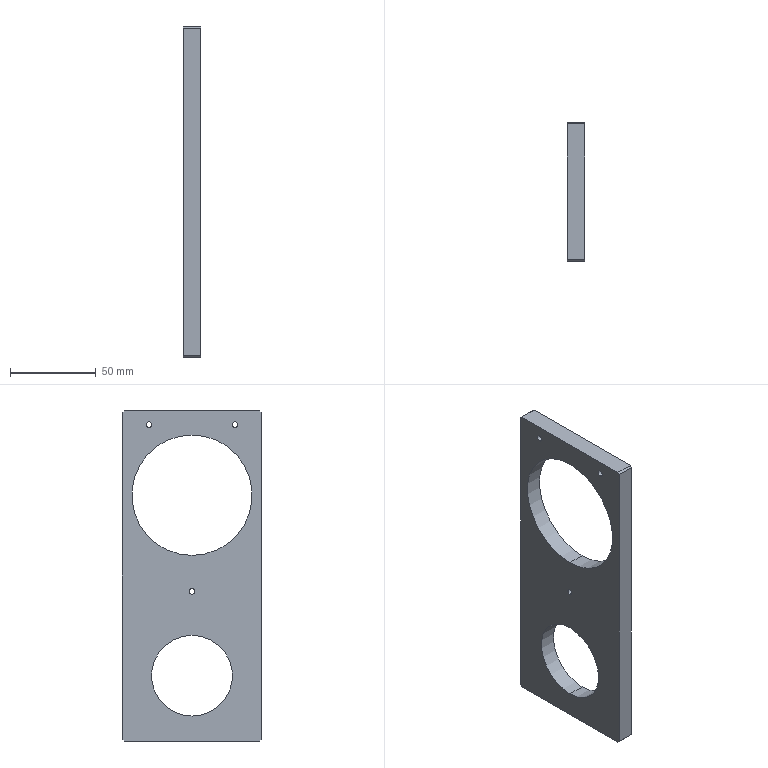Part | STEP file | FFH80-PL-008^FFH85-PL-M75-B3-01_three-axis module | 1 solid | 20 faces | box 10 x 81 x 192 mm | volume 99409 mm3 | cylinder 10 | plane 10 | commonest cylinder face diameters 3.3 x6 47 x2 70 x2
STEP:
#1=CARTESIAN_POINT('',(0.,25.,89.65));
#2=VERTEX_POINT('',#1);
#3=CARTESIAN_POINT('',(0.,25.,86.35));
#4=VERTEX_POINT('',#3);
#5=CARTESIAN_POINT('',(0.,25.,88.));
#6=DIRECTION('',(1.,0.,0.));
#7=DIRECTION('',(0.,0.,-1.));
#8=AXIS2_PLACEMENT_3D('',#5,#6,#7);
#9=CIRCLE('',#8,1.65);
#10=EDGE_CURVE('',#2,#4,#9,.T.);
#11=ORIENTED_EDGE('',*,*,#10,.F.);
#12=CARTESIAN_POINT('',(10.,25.,89.65));
#13=VERTEX_POINT('',#12);
#14=CARTESIAN_POINT('',(10.,25.,89.65));
#15=DIRECTION('',(1.,0.,0.));
#16=VECTOR('',#15,1000.);
#17=LINE('',#14,#16);
#18=EDGE_CURVE('',#2,#13,#17,.T.);
#19=ORIENTED_EDGE('',*,*,#18,.T.);
#20=CARTESIAN_POINT('',(10.,25.,86.35));
#21=VERTEX_POINT('',#20);
#22=CARTESIAN_POINT('',(10.,25.,88.));
#23=DIRECTION('',(-1.,0.,0.));
#24=DIRECTION('',(0.,0.,-1.));
#25=AXIS2_PLACEMENT_3D('',#22,#23,#24);
#26=CIRCLE('',#25,1.65);
#27=EDGE_CURVE('',#21,#13,#26,.T.);
#28=ORIENTED_EDGE('',*,*,#27,.F.);
#29=CARTESIAN_POINT('',(10.,25.,86.35));
#30=DIRECTION('',(1.,0.,0.));
#31=VECTOR('',#30,1000.);
#32=LINE('',#29,#31);
#33=EDGE_CURVE('',#4,#21,#32,.T.);
#34=ORIENTED_EDGE('',*,*,#33,.F.);
#35=EDGE_LOOP('',(#11,#19,#28,#34));
#36=FACE_OUTER_BOUND('',#35,.T.);
#37=CARTESIAN_POINT('',(10.,25.,88.));
#38=DIRECTION('',(1.,0.,0.));
#39=DIRECTION('',(0.,0.,-1.));
#40=AXIS2_PLACEMENT_3D('',#37,#38,#39);
#41=CYLINDRICAL_SURFACE('',#40,1.65);
#42=ADVANCED_FACE('',(#36),#41,.F.);
#43=CARTESIAN_POINT('',(0.,0.,-7.35));
#44=VERTEX_POINT('',#43);
#45=CARTESIAN_POINT('',(0.,0.,-10.65));
#46=VERTEX_POINT('',#45);
#47=CARTESIAN_POINT('',(0.,0.,-9.));
#48=DIRECTION('',(1.,0.,0.));
#49=DIRECTION('',(0.,0.,-1.));
#50=AXIS2_PLACEMENT_3D('',#47,#48,#49);
#51=CIRCLE('',#50,1.65);
#52=EDGE_CURVE('',#44,#46,#51,.T.);
#53=ORIENTED_EDGE('',*,*,#52,.F.);
#54=CARTESIAN_POINT('',(10.,0.,-7.35));
#55=VERTEX_POINT('',#54);
#56=CARTESIAN_POINT('',(10.,0.,-7.35));
#57=DIRECTION('',(1.,0.,0.));
#58=VECTOR('',#57,1000.);
#59=LINE('',#56,#58);
#60=EDGE_CURVE('',#44,#55,#59,.T.);
#61=ORIENTED_EDGE('',*,*,#60,.T.);
#62=CARTESIAN_POINT('',(10.,0.,-10.65));
#63=VERTEX_POINT('',#62);
#64=CARTESIAN_POINT('',(10.,0.,-9.));
#65=DIRECTION('',(-1.,0.,0.));
#66=DIRECTION('',(0.,0.,-1.));
#67=AXIS2_PLACEMENT_3D('',#64,#65,#66);
#68=CIRCLE('',#67,1.65);
#69=EDGE_CURVE('',#63,#55,#68,.T.);
#70=ORIENTED_EDGE('',*,*,#69,.F.);
#71=CARTESIAN_POINT('',(10.,0.,-10.65));
#72=DIRECTION('',(1.,0.,0.));
#73=VECTOR('',#72,1000.);
#74=LINE('',#71,#73);
#75=EDGE_CURVE('',#46,#63,#74,.T.);
#76=ORIENTED_EDGE('',*,*,#75,.F.);
#77=EDGE_LOOP('',(#53,#61,#70,#76));
#78=FACE_OUTER_BOUND('',#77,.T.);
#79=CARTESIAN_POINT('',(10.,0.,-9.));
#80=DIRECTION('',(1.,0.,0.));
#81=DIRECTION('',(0.,0.,-1.));
#82=AXIS2_PLACEMENT_3D('',#79,#80,#81);
#83=CYLINDRICAL_SURFACE('',#82,1.65);
#84=ADVANCED_FACE('',(#78),#83,.F.);
#85=CARTESIAN_POINT('',(0.,-25.,89.65));
#86=VERTEX_POINT('',#85);
#87=CARTESIAN_POINT('',(0.,-25.,86.35));
#88=VERTEX_POINT('',#87);
#89=CARTESIAN_POINT('',(0.,-25.,88.));
#90=DIRECTION('',(1.,0.,0.));
#91=DIRECTION('',(0.,0.,-1.));
#92=AXIS2_PLACEMENT_3D('',#89,#90,#91);
#93=CIRCLE('',#92,1.65);
#94=EDGE_CURVE('',#86,#88,#93,.T.);
#95=ORIENTED_EDGE('',*,*,#94,.F.);
#96=CARTESIAN_POINT('',(10.,-25.,89.65));
#97=VERTEX_POINT('',#96);
#98=CARTESIAN_POINT('',(10.,-25.,89.65));
#99=DIRECTION('',(1.,0.,0.));
#100=VECTOR('',#99,1000.);
#101=LINE('',#98,#100);
#102=EDGE_CURVE('',#86,#97,#101,.T.);
#103=ORIENTED_EDGE('',*,*,#102,.T.);
#104=CARTESIAN_POINT('',(10.,-25.,86.35));
#105=VERTEX_POINT('',#104);
#106=CARTESIAN_POINT('',(10.,-25.,88.));
#107=DIRECTION('',(-1.,0.,0.));
#108=DIRECTION('',(0.,0.,-1.));
#109=AXIS2_PLACEMENT_3D('',#106,#107,#108);
#110=CIRCLE('',#109,1.65);
#111=EDGE_CURVE('',#105,#97,#110,.T.);
#112=ORIENTED_EDGE('',*,*,#111,.F.);
#113=CARTESIAN_POINT('',(10.,-25.,86.35));
#114=DIRECTION('',(1.,0.,0.));
#115=VECTOR('',#114,1000.);
#116=LINE('',#113,#115);
#117=EDGE_CURVE('',#88,#105,#116,.T.);
#118=ORIENTED_EDGE('',*,*,#117,.F.);
#119=EDGE_LOOP('',(#95,#103,#112,#118));
#120=FACE_OUTER_BOUND('',#119,.T.);
#121=CARTESIAN_POINT('',(10.,-25.,88.));
#122=DIRECTION('',(1.,0.,0.));
#123=DIRECTION('',(0.,0.,-1.));
#124=AXIS2_PLACEMENT_3D('',#121,#122,#123);
#125=CYLINDRICAL_SURFACE('',#124,1.65);
#126=ADVANCED_FACE('',(#120),#125,.F.);
#127=CARTESIAN_POINT('',(0.,0.,82.));
#128=VERTEX_POINT('',#127);
#129=CARTESIAN_POINT('',(0.,0.,12.));
#130=VERTEX_POINT('',#129);
#131=CARTESIAN_POINT('',(0.,0.,47.));
#132=DIRECTION('',(1.,0.,0.));
#133=DIRECTION('',(0.,0.,-1.));
#134=AXIS2_PLACEMENT_3D('',#131,#132,#133);
#135=CIRCLE('',#134,35.);
#136=EDGE_CURVE('',#128,#130,#135,.T.);
#137=ORIENTED_EDGE('',*,*,#136,.F.);
#138=CARTESIAN_POINT('',(10.,0.,82.));
#139=VERTEX_POINT('',#138);
#140=CARTESIAN_POINT('',(0.,0.,82.));
#141=DIRECTION('',(1.,0.,0.));
#142=VECTOR('',#141,1000.);
#143=LINE('',#140,#142);
#144=EDGE_CURVE('',#128,#139,#143,.T.);
#145=ORIENTED_EDGE('',*,*,#144,.T.);
#146=CARTESIAN_POINT('',(10.,0.,12.));
#147=VERTEX_POINT('',#146);
#148=CARTESIAN_POINT('',(10.,0.,47.));
#149=DIRECTION('',(-1.,0.,0.));
#150=DIRECTION('',(0.,0.,-1.));
#151=AXIS2_PLACEMENT_3D('',#148,#149,#150);
#152=CIRCLE('',#151,35.);
#153=EDGE_CURVE('',#147,#139,#152,.T.);
#154=ORIENTED_EDGE('',*,*,#153,.F.);
#155=CARTESIAN_POINT('',(0.,0.,12.));
#156=DIRECTION('',(1.,0.,0.));
#157=VECTOR('',#156,1000.);
#158=LINE('',#155,#157);
#159=EDGE_CURVE('',#130,#147,#158,.T.);
#160=ORIENTED_EDGE('',*,*,#159,.F.);
#161=EDGE_LOOP('',(#137,#145,#154,#160));
#162=FACE_OUTER_BOUND('',#161,.T.);
#163=CARTESIAN_POINT('',(0.,0.,47.));
#164=DIRECTION('',(1.,0.,0.));
#165=DIRECTION('',(0.,0.,-1.));
#166=AXIS2_PLACEMENT_3D('',#163,#164,#165);
#167=CYLINDRICAL_SURFACE('',#166,35.);
#168=ADVANCED_FACE('',(#162),#167,.F.);
#169=CARTESIAN_POINT('',(0.,0.,-34.5));
#170=VERTEX_POINT('',#169);
#171=CARTESIAN_POINT('',(0.,0.,-81.5));
#172=VERTEX_POINT('',#171);
#173=CARTESIAN_POINT('',(0.,0.,-58.));
#174=DIRECTION('',(1.,0.,0.));
#175=DIRECTION('',(0.,0.,-1.));
#176=AXIS2_PLACEMENT_3D('',#173,#174,#175);
#177=CIRCLE('',#176,23.5);
#178=EDGE_CURVE('',#170,#172,#177,.T.);
#179=ORIENTED_EDGE('',*,*,#178,.F.);
#180=CARTESIAN_POINT('',(10.,0.,-34.5));
#181=VERTEX_POINT('',#180);
#182=CARTESIAN_POINT('',(0.,0.,-34.5));
#183=DIRECTION('',(1.,0.,0.));
#184=VECTOR('',#183,1000.);
#185=LINE('',#182,#184);
#186=EDGE_CURVE('',#170,#181,#185,.T.);
#187=ORIENTED_EDGE('',*,*,#186,.T.);
#188=CARTESIAN_POINT('',(10.,0.,-81.5));
#189=VERTEX_POINT('',#188);
#190=CARTESIAN_POINT('',(10.,0.,-58.));
#191=DIRECTION('',(-1.,0.,0.));
#192=DIRECTION('',(0.,0.,-1.));
#193=AXIS2_PLACEMENT_3D('',#190,#191,#192);
#194=CIRCLE('',#193,23.5);
#195=EDGE_CURVE('',#189,#181,#194,.T.);
#196=ORIENTED_EDGE('',*,*,#195,.F.);
#197=CARTESIAN_POINT('',(0.,0.,-81.5));
#198=DIRECTION('',(1.,0.,0.));
#199=VECTOR('',#198,1000.);
#200=LINE('',#197,#199);
#201=EDGE_CURVE('',#172,#189,#200,.T.);
#202=ORIENTED_EDGE('',*,*,#201,.F.);
#203=EDGE_LOOP('',(#179,#187,#196,#202));
#204=FACE_OUTER_BOUND('',#203,.T.);
#205=CARTESIAN_POINT('',(0.,0.,-58.));
#206=DIRECTION('',(1.,0.,0.));
#207=DIRECTION('',(0.,0.,-1.));
#208=AXIS2_PLACEMENT_3D('',#205,#206,#207);
#209=CYLINDRICAL_SURFACE('',#208,23.5);
#210=ADVANCED_FACE('',(#204),#209,.F.);
#211=CARTESIAN_POINT('',(0.,25.,88.));
#212=DIRECTION('',(1.,0.,0.));
#213=DIRECTION('',(0.,0.,-1.));
#214=AXIS2_PLACEMENT_3D('',#211,#212,#213);
#215=CIRCLE('',#214,1.65);
#216=EDGE_CURVE('',#4,#2,#215,.T.);
#217=ORIENTED_EDGE('',*,*,#216,.T.);
#218=ORIENTED_EDGE('',*,*,#10,.T.);
#219=EDGE_LOOP('',(#217,#218));
#220=FACE_BOUND('',#219,.T.);
#221=CARTESIAN_POINT('',(0.,0.,-9.));
#222=DIRECTION('',(1.,0.,0.));
#223=DIRECTION('',(0.,0.,-1.));
#224=AXIS2_PLACEMENT_3D('',#221,#222,#223);
#225=CIRCLE('',#224,1.65);
#226=EDGE_CURVE('',#46,#44,#225,.T.);
#227=ORIENTED_EDGE('',*,*,#226,.T.);
#228=ORIENTED_EDGE('',*,*,#52,.T.);
#229=EDGE_LOOP('',(#227,#228));
#230=FACE_BOUND('',#229,.T.);
#231=CARTESIAN_POINT('',(0.,-25.,88.));
#232=DIRECTION('',(1.,0.,0.));
#233=DIRECTION('',(0.,0.,-1.));
#234=AXIS2_PLACEMENT_3D('',#231,#232,#233);
#235=CIRCLE('',#234,1.65);
#236=EDGE_CURVE('',#88,#86,#235,.T.);
#237=ORIENTED_EDGE('',*,*,#236,.T.);
#238=ORIENTED_EDGE('',*,*,#94,.T.);
#239=EDGE_LOOP('',(#237,#238));
#240=FACE_BOUND('',#239,.T.);
#241=CARTESIAN_POINT('',(0.,0.,47.));
#242=DIRECTION('',(1.,0.,0.));
#243=DIRECTION('',(0.,0.,-1.));
#244=AXIS2_PLACEMENT_3D('',#241,#242,#243);
#245=CIRCLE('',#244,35.);
#246=EDGE_CURVE('',#130,#128,#245,.T.);
#247=ORIENTED_EDGE('',*,*,#246,.T.);
#248=ORIENTED_EDGE('',*,*,#136,.T.);
#249=EDGE_LOOP('',(#247,#248));
#250=FACE_BOUND('',#249,.T.);
#251=CARTESIAN_POINT('',(0.,0.,-58.));
#252=DIRECTION('',(1.,0.,0.));
#253=DIRECTION('',(0.,0.,-1.));
#254=AXIS2_PLACEMENT_3D('',#251,#252,#253);
#255=CIRCLE('',#254,23.5);
#256=EDGE_CURVE('',#172,#170,#255,.T.);
#257=ORIENTED_EDGE('',*,*,#256,.T.);
#258=ORIENTED_EDGE('',*,*,#178,.T.);
#259=EDGE_LOOP('',(#257,#258));
#260=FACE_BOUND('',#259,.T.);
#261=CARTESIAN_POINT('',(0.,-40.5,-95.));
#262=VERTEX_POINT('',#261);
#263=CARTESIAN_POINT('',(0.,-40.5,95.));
#264=VERTEX_POINT('',#263);
#265=CARTESIAN_POINT('',(0.,-40.5,0.));
#266=DIRECTION('',(0.,0.,1.));
#267=VECTOR('',#266,1000.);
#268=LINE('',#265,#267);
#269=EDGE_CURVE('',#262,#264,#268,.T.);
#270=ORIENTED_EDGE('',*,*,#269,.T.);
#271=CARTESIAN_POINT('',(0.,-39.5,96.));
#272=VERTEX_POINT('',#271);
#273=CARTESIAN_POINT('',(0.,-40.5,95.));
#274=DIRECTION('',(0.,0.7071,0.7071));
#275=VECTOR('',#274,1000.);
#276=LINE('',#273,#275);
#277=EDGE_CURVE('',#264,#272,#276,.T.);
#278=ORIENTED_EDGE('',*,*,#277,.T.);
#279=CARTESIAN_POINT('',(0.,39.5,96.));
#280=VERTEX_POINT('',#279);
#281=CARTESIAN_POINT('',(0.,0.,96.));
#282=DIRECTION('',(0.,1.,0.));
#283=VECTOR('',#282,1000.);
#284=LINE('',#281,#283);
#285=EDGE_CURVE('',#272,#280,#284,.T.);
#286=ORIENTED_EDGE('',*,*,#285,.T.);
#287=CARTESIAN_POINT('',(0.,40.5,95.));
#288=VERTEX_POINT('',#287);
#289=CARTESIAN_POINT('',(0.,39.5,96.));
#290=DIRECTION('',(0.,0.7071,-0.7071));
#291=VECTOR('',#290,1000.);
#292=LINE('',#289,#291);
#293=EDGE_CURVE('',#280,#288,#292,.T.);
#294=ORIENTED_EDGE('',*,*,#293,.T.);
#295=CARTESIAN_POINT('',(0.,40.5,-95.));
#296=VERTEX_POINT('',#295);
#297=CARTESIAN_POINT('',(0.,40.5,0.));
#298=DIRECTION('',(0.,0.,-1.));
#299=VECTOR('',#298,1000.);
#300=LINE('',#297,#299);
#301=EDGE_CURVE('',#288,#296,#300,.T.);
#302=ORIENTED_EDGE('',*,*,#301,.T.);
#303=CARTESIAN_POINT('',(0.,39.5,-96.));
#304=VERTEX_POINT('',#303);
#305=CARTESIAN_POINT('',(0.,40.5,-95.));
#306=DIRECTION('',(0.,-0.7071,-0.7071));
#307=VECTOR('',#306,1000.);
#308=LINE('',#305,#307);
#309=EDGE_CURVE('',#296,#304,#308,.T.);
#310=ORIENTED_EDGE('',*,*,#309,.T.);
#311=CARTESIAN_POINT('',(0.,-39.5,-96.));
#312=VERTEX_POINT('',#311);
#313=CARTESIAN_POINT('',(0.,0.,-96.));
#314=DIRECTION('',(0.,-1.,0.));
#315=VECTOR('',#314,1000.);
#316=LINE('',#313,#315);
#317=EDGE_CURVE('',#304,#312,#316,.T.);
#318=ORIENTED_EDGE('',*,*,#317,.T.);
#319=CARTESIAN_POINT('',(0.,-39.5,-96.));
#320=DIRECTION('',(0.,-0.7071,0.7071));
#321=VECTOR('',#320,1000.);
#322=LINE('',#319,#321);
#323=EDGE_CURVE('',#312,#262,#322,.T.);
#324=ORIENTED_EDGE('',*,*,#323,.T.);
#325=EDGE_LOOP('',(#270,#278,#286,#294,#302,#310,#318,#324));
#326=FACE_OUTER_BOUND('',#325,.T.);
#327=CARTESIAN_POINT('',(0.,0.,0.));
#328=DIRECTION('',(-1.,0.,0.));
#329=DIRECTION('',(0.,0.,1.));
#330=AXIS2_PLACEMENT_3D('',#327,#328,#329);
#331=PLANE('',#330);
#332=ADVANCED_FACE('',(#220,#230,#240,#250,#260,#326),#331,.T.);
#333=ORIENTED_EDGE('',*,*,#18,.F.);
#334=ORIENTED_EDGE('',*,*,#216,.F.);
#335=ORIENTED_EDGE('',*,*,#33,.T.);
#336=CARTESIAN_POINT('',(10.,25.,88.));
#337=DIRECTION('',(-1.,0.,0.));
#338=DIRECTION('',(0.,0.,-1.));
#339=AXIS2_PLACEMENT_3D('',#336,#337,#338);
#340=CIRCLE('',#339,1.65);
#341=EDGE_CURVE('',#13,#21,#340,.T.);
#342=ORIENTED_EDGE('',*,*,#341,.F.);
#343=EDGE_LOOP('',(#333,#334,#335,#342));
#344=FACE_OUTER_BOUND('',#343,.T.);
#345=CARTESIAN_POINT('',(10.,25.,88.));
#346=DIRECTION('',(1.,0.,0.));
#347=DIRECTION('',(0.,0.,-1.));
#348=AXIS2_PLACEMENT_3D('',#345,#346,#347);
#349=CYLINDRICAL_SURFACE('',#348,1.65);
#350=ADVANCED_FACE('',(#344),#349,.F.);
#351=ORIENTED_EDGE('',*,*,#60,.F.);
#352=ORIENTED_EDGE('',*,*,#226,.F.);
#353=ORIENTED_EDGE('',*,*,#75,.T.);
#354=CARTESIAN_POINT('',(10.,0.,-9.));
#355=DIRECTION('',(-1.,0.,0.));
#356=DIRECTION('',(0.,0.,-1.));
#357=AXIS2_PLACEMENT_3D('',#354,#355,#356);
#358=CIRCLE('',#357,1.65);
#359=EDGE_CURVE('',#55,#63,#358,.T.);
#360=ORIENTED_EDGE('',*,*,#359,.F.);
#361=EDGE_LOOP('',(#351,#352,#353,#360));
#362=FACE_OUTER_BOUND('',#361,.T.);
#363=CARTESIAN_POINT('',(10.,0.,-9.));
#364=DIRECTION('',(1.,0.,0.));
#365=DIRECTION('',(0.,0.,-1.));
#366=AXIS2_PLACEMENT_3D('',#363,#364,#365);
#367=CYLINDRICAL_SURFACE('',#366,1.65);
#368=ADVANCED_FACE('',(#362),#367,.F.);
#369=ORIENTED_EDGE('',*,*,#102,.F.);
#370=ORIENTED_EDGE('',*,*,#236,.F.);
#371=ORIENTED_EDGE('',*,*,#117,.T.);
#372=CARTESIAN_POINT('',(10.,-25.,88.));
#373=DIRECTION('',(-1.,0.,0.));
#374=DIRECTION('',(0.,0.,-1.));
#375=AXIS2_PLACEMENT_3D('',#372,#373,#374);
#376=CIRCLE('',#375,1.65);
#377=EDGE_CURVE('',#97,#105,#376,.T.);
#378=ORIENTED_EDGE('',*,*,#377,.F.);
#379=EDGE_LOOP('',(#369,#370,#371,#378));
#380=FACE_OUTER_BOUND('',#379,.T.);
#381=CARTESIAN_POINT('',(10.,-25.,88.));
#382=DIRECTION('',(1.,0.,0.));
#383=DIRECTION('',(0.,0.,-1.));
#384=AXIS2_PLACEMENT_3D('',#381,#382,#383);
#385=CYLINDRICAL_SURFACE('',#384,1.65);
#386=ADVANCED_FACE('',(#380),#385,.F.);
#387=ORIENTED_EDGE('',*,*,#144,.F.);
#388=ORIENTED_EDGE('',*,*,#246,.F.);
#389=ORIENTED_EDGE('',*,*,#159,.T.);
#390=CARTESIAN_POINT('',(10.,0.,47.));
#391=DIRECTION('',(-1.,0.,0.));
#392=DIRECTION('',(0.,0.,-1.));
#393=AXIS2_PLACEMENT_3D('',#390,#391,#392);
#394=CIRCLE('',#393,35.);
#395=EDGE_CURVE('',#139,#147,#394,.T.);
#396=ORIENTED_EDGE('',*,*,#395,.F.);
#397=EDGE_LOOP('',(#387,#388,#389,#396));
#398=FACE_OUTER_BOUND('',#397,.T.);
#399=CARTESIAN_POINT('',(0.,0.,47.));
#400=DIRECTION('',(1.,0.,0.));
#401=DIRECTION('',(0.,0.,-1.));
#402=AXIS2_PLACEMENT_3D('',#399,#400,#401);
#403=CYLINDRICAL_SURFACE('',#402,35.);
#404=ADVANCED_FACE('',(#398),#403,.F.);
#405=ORIENTED_EDGE('',*,*,#186,.F.);
#406=ORIENTED_EDGE('',*,*,#256,.F.);
#407=ORIENTED_EDGE('',*,*,#201,.T.);
#408=CARTESIAN_POINT('',(10.,0.,-58.));
#409=DIRECTION('',(-1.,0.,0.));
#410=DIRECTION('',(0.,0.,-1.));
#411=AXIS2_PLACEMENT_3D('',#408,#409,#410);
#412=CIRCLE('',#411,23.5);
#413=EDGE_CURVE('',#181,#189,#412,.T.);
#414=ORIENTED_EDGE('',*,*,#413,.F.);
#415=EDGE_LOOP('',(#405,#406,#407,#414));
#416=FACE_OUTER_BOUND('',#415,.T.);
#417=CARTESIAN_POINT('',(0.,0.,-58.));
#418=DIRECTION('',(1.,0.,0.));
#419=DIRECTION('',(0.,0.,-1.));
#420=AXIS2_PLACEMENT_3D('',#417,#418,#419);
#421=CYLINDRICAL_SURFACE('',#420,23.5);
#422=ADVANCED_FACE('',(#416),#421,.F.);
#423=CARTESIAN_POINT('',(10.,-40.5,95.));
#424=VERTEX_POINT('',#423);
#425=CARTESIAN_POINT('',(10.,-40.5,-95.));
#426=VERTEX_POINT('',#425);
#427=CARTESIAN_POINT('',(10.,-40.5,-96.));
#428=DIRECTION('',(0.,0.,-1.));
#429=VECTOR('',#428,1000.);
#430=LINE('',#427,#429);
#431=EDGE_CURVE('',#424,#426,#430,.T.);
#432=ORIENTED_EDGE('',*,*,#431,.F.);
#433=CARTESIAN_POINT('',(10.,-40.5,95.));
#434=DIRECTION('',(1.,0.,0.));
#435=VECTOR('',#434,1000.);
#436=LINE('',#433,#435);
#437=EDGE_CURVE('',#264,#424,#436,.T.);
#438=ORIENTED_EDGE('',*,*,#437,.F.);
#439=ORIENTED_EDGE('',*,*,#269,.F.);
#440=CARTESIAN_POINT('',(10.,-40.5,-95.));
#441=DIRECTION('',(-1.,0.,0.));
#442=VECTOR('',#441,1000.);
#443=LINE('',#440,#442);
#444=EDGE_CURVE('',#426,#262,#443,.T.);
#445=ORIENTED_EDGE('',*,*,#444,.F.);
#446=EDGE_LOOP('',(#432,#438,#439,#445));
#447=FACE_OUTER_BOUND('',#446,.T.);
#448=CARTESIAN_POINT('',(10.,-40.5,-96.));
#449=DIRECTION('',(0.,1.,0.));
#450=DIRECTION('',(0.,0.,1.));
#451=AXIS2_PLACEMENT_3D('',#448,#449,#450);
#452=PLANE('',#451);
#453=ADVANCED_FACE('',(#447),#452,.F.);
#454=CARTESIAN_POINT('',(10.,-39.5,-96.));
#455=VERTEX_POINT('',#454);
#456=CARTESIAN_POINT('',(10.,39.5,-96.));
#457=VERTEX_POINT('',#456);
#458=CARTESIAN_POINT('',(10.,40.5,-96.));
#459=DIRECTION('',(0.,1.,0.));
#460=VECTOR('',#459,1000.);
#461=LINE('',#458,#460);
#462=EDGE_CURVE('',#455,#457,#461,.T.);
#463=ORIENTED_EDGE('',*,*,#462,.F.);
#464=CARTESIAN_POINT('',(10.,-39.5,-96.));
#465=DIRECTION('',(1.,0.,0.));
#466=VECTOR('',#465,1000.);
#467=LINE('',#464,#466);
#468=EDGE_CURVE('',#312,#455,#467,.T.);
#469=ORIENTED_EDGE('',*,*,#468,.F.);
#470=ORIENTED_EDGE('',*,*,#317,.F.);
#471=CARTESIAN_POINT('',(10.,39.5,-96.));
#472=DIRECTION('',(-1.,0.,0.));
#473=VECTOR('',#472,1000.);
#474=LINE('',#471,#473);
#475=EDGE_CURVE('',#457,#304,#474,.T.);
#476=ORIENTED_EDGE('',*,*,#475,.F.);
#477=EDGE_LOOP('',(#463,#469,#470,#476));
#478=FACE_OUTER_BOUND('',#477,.T.);
#479=CARTESIAN_POINT('',(10.,40.5,-96.));
#480=DIRECTION('',(0.,0.,1.));
#481=DIRECTION('',(0.,-1.,0.));
#482=AXIS2_PLACEMENT_3D('',#479,#480,#481);
#483=PLANE('',#482);
#484=ADVANCED_FACE('',(#478),#483,.F.);
#485=ORIENTED_EDGE('',*,*,#301,.F.);
#486=CARTESIAN_POINT('',(10.,40.5,95.));
#487=VERTEX_POINT('',#486);
#488=CARTESIAN_POINT('',(10.,40.5,95.));
#489=DIRECTION('',(-1.,0.,0.));
#490=VECTOR('',#489,1000.);
#491=LINE('',#488,#490);
#492=EDGE_CURVE('',#487,#288,#491,.T.);
#493=ORIENTED_EDGE('',*,*,#492,.F.);
#494=CARTESIAN_POINT('',(10.,40.5,-95.));
#495=VERTEX_POINT('',#494);
#496=CARTESIAN_POINT('',(10.,40.5,-96.));
#497=DIRECTION('',(0.,0.,1.));
#498=VECTOR('',#497,1000.);
#499=LINE('',#496,#498);
#500=EDGE_CURVE('',#495,#487,#499,.T.);
#501=ORIENTED_EDGE('',*,*,#500,.F.);
#502=CARTESIAN_POINT('',(10.,40.5,-95.));
#503=DIRECTION('',(1.,0.,0.));
#504=VECTOR('',#503,1000.);
#505=LINE('',#502,#504);
#506=EDGE_CURVE('',#296,#495,#505,.T.);
#507=ORIENTED_EDGE('',*,*,#506,.F.);
#508=EDGE_LOOP('',(#485,#493,#501,#507));
#509=FACE_OUTER_BOUND('',#508,.T.);
#510=CARTESIAN_POINT('',(10.,40.5,-96.));
#511=DIRECTION('',(0.,-1.,0.));
#512=DIRECTION('',(0.,0.,-1.));
#513=AXIS2_PLACEMENT_3D('',#510,#511,#512);
#514=PLANE('',#513);
#515=ADVANCED_FACE('',(#509),#514,.F.);
#516=CARTESIAN_POINT('',(10.,39.5,96.));
#517=VERTEX_POINT('',#516);
#518=CARTESIAN_POINT('',(10.,-39.5,96.));
#519=VERTEX_POINT('',#518);
#520=CARTESIAN_POINT('',(10.,40.5,96.));
#521=DIRECTION('',(0.,-1.,0.));
#522=VECTOR('',#521,1000.);
#523=LINE('',#520,#522);
#524=EDGE_CURVE('',#517,#519,#523,.T.);
#525=ORIENTED_EDGE('',*,*,#524,.F.);
#526=CARTESIAN_POINT('',(10.,39.5,96.));
#527=DIRECTION('',(1.,0.,0.));
#528=VECTOR('',#527,1000.);
#529=LINE('',#526,#528);
#530=EDGE_CURVE('',#280,#517,#529,.T.);
#531=ORIENTED_EDGE('',*,*,#530,.F.);
#532=ORIENTED_EDGE('',*,*,#285,.F.);
#533=CARTESIAN_POINT('',(10.,-39.5,96.));
#534=DIRECTION('',(-1.,0.,0.));
#535=VECTOR('',#534,1000.);
#536=LINE('',#533,#535);
#537=EDGE_CURVE('',#519,#272,#536,.T.);
#538=ORIENTED_EDGE('',*,*,#537,.F.);
#539=EDGE_LOOP('',(#525,#531,#532,#538));
#540=FACE_OUTER_BOUND('',#539,.T.);
#541=CARTESIAN_POINT('',(10.,40.5,96.));
#542=DIRECTION('',(0.,0.,-1.));
#543=DIRECTION('',(0.,1.,0.));
#544=AXIS2_PLACEMENT_3D('',#541,#542,#543);
#545=PLANE('',#544);
#546=ADVANCED_FACE('',(#540),#545,.F.);
#547=ORIENTED_EDGE('',*,*,#27,.T.);
#548=ORIENTED_EDGE('',*,*,#341,.T.);
#549=EDGE_LOOP('',(#547,#548));
#550=FACE_BOUND('',#549,.T.);
#551=ORIENTED_EDGE('',*,*,#69,.T.);
#552=ORIENTED_EDGE('',*,*,#359,.T.);
#553=EDGE_LOOP('',(#551,#552));
#554=FACE_BOUND('',#553,.T.);
#555=ORIENTED_EDGE('',*,*,#111,.T.);
#556=ORIENTED_EDGE('',*,*,#377,.T.);
#557=EDGE_LOOP('',(#555,#556));
#558=FACE_BOUND('',#557,.T.);
#559=ORIENTED_EDGE('',*,*,#153,.T.);
#560=ORIENTED_EDGE('',*,*,#395,.T.);
#561=EDGE_LOOP('',(#559,#560));
#562=FACE_BOUND('',#561,.T.);
#563=ORIENTED_EDGE('',*,*,#195,.T.);
#564=ORIENTED_EDGE('',*,*,#413,.T.);
#565=EDGE_LOOP('',(#563,#564));
#566=FACE_BOUND('',#565,.T.);
#567=ORIENTED_EDGE('',*,*,#500,.T.);
#568=CARTESIAN_POINT('',(10.,39.5,96.));
#569=DIRECTION('',(0.,0.7071,-0.7071));
#570=VECTOR('',#569,1000.);
#571=LINE('',#568,#570);
#572=EDGE_CURVE('',#517,#487,#571,.T.);
#573=ORIENTED_EDGE('',*,*,#572,.F.);
#574=ORIENTED_EDGE('',*,*,#524,.T.);
#575=CARTESIAN_POINT('',(10.,-40.5,95.));
#576=DIRECTION('',(0.,0.7071,0.7071));
#577=VECTOR('',#576,1000.);
#578=LINE('',#575,#577);
#579=EDGE_CURVE('',#424,#519,#578,.T.);
#580=ORIENTED_EDGE('',*,*,#579,.F.);
#581=ORIENTED_EDGE('',*,*,#431,.T.);
#582=CARTESIAN_POINT('',(10.,-39.5,-96.));
#583=DIRECTION('',(0.,-0.7071,0.7071));
#584=VECTOR('',#583,1000.);
#585=LINE('',#582,#584);
#586=EDGE_CURVE('',#455,#426,#585,.T.);
#587=ORIENTED_EDGE('',*,*,#586,.F.);
#588=ORIENTED_EDGE('',*,*,#462,.T.);
#589=CARTESIAN_POINT('',(10.,40.5,-95.));
#590=DIRECTION('',(0.,-0.7071,-0.7071));
#591=VECTOR('',#590,1000.);
#592=LINE('',#589,#591);
#593=EDGE_CURVE('',#495,#457,#592,.T.);
#594=ORIENTED_EDGE('',*,*,#593,.F.);
#595=EDGE_LOOP('',(#567,#573,#574,#580,#581,#587,#588,#594));
#596=FACE_OUTER_BOUND('',#595,.T.);
#597=CARTESIAN_POINT('',(10.,0.,0.));
#598=DIRECTION('',(-1.,0.,0.));
#599=DIRECTION('',(0.,0.,1.));
#600=AXIS2_PLACEMENT_3D('',#597,#598,#599);
#601=PLANE('',#600);
#602=ADVANCED_FACE('',(#550,#554,#558,#562,#566,#596),#601,.F.);
#603=ORIENTED_EDGE('',*,*,#323,.F.);
#604=ORIENTED_EDGE('',*,*,#468,.T.);
#605=ORIENTED_EDGE('',*,*,#586,.T.);
#606=ORIENTED_EDGE('',*,*,#444,.T.);
#607=EDGE_LOOP('',(#603,#604,#605,#606));
#608=FACE_OUTER_BOUND('',#607,.T.);
#609=CARTESIAN_POINT('',(10.,-39.5,-96.));
#610=DIRECTION('',(0.,0.7071,0.7071));
#611=DIRECTION('',(0.,-0.7071,0.7071));
#612=AXIS2_PLACEMENT_3D('',#609,#610,#611);
#613=PLANE('',#612);
#614=ADVANCED_FACE('',(#608),#613,.F.);
#615=ORIENTED_EDGE('',*,*,#277,.F.);
#616=ORIENTED_EDGE('',*,*,#437,.T.);
#617=ORIENTED_EDGE('',*,*,#579,.T.);
#618=ORIENTED_EDGE('',*,*,#537,.T.);
#619=EDGE_LOOP('',(#615,#616,#617,#618));
#620=FACE_OUTER_BOUND('',#619,.T.);
#621=CARTESIAN_POINT('',(10.,-40.5,95.));
#622=DIRECTION('',(0.,0.7071,-0.7071));
#623=DIRECTION('',(0.,0.7071,0.7071));
#624=AXIS2_PLACEMENT_3D('',#621,#622,#623);
#625=PLANE('',#624);
#626=ADVANCED_FACE('',(#620),#625,.F.);
#627=ORIENTED_EDGE('',*,*,#309,.F.);
#628=ORIENTED_EDGE('',*,*,#506,.T.);
#629=ORIENTED_EDGE('',*,*,#593,.T.);
#630=ORIENTED_EDGE('',*,*,#475,.T.);
#631=EDGE_LOOP('',(#627,#628,#629,#630));
#632=FACE_OUTER_BOUND('',#631,.T.);
#633=CARTESIAN_POINT('',(10.,40.5,-95.));
#634=DIRECTION('',(0.,-0.7071,0.7071));
#635=DIRECTION('',(0.,-0.7071,-0.7071));
#636=AXIS2_PLACEMENT_3D('',#633,#634,#635);
#637=PLANE('',#636);
#638=ADVANCED_FACE('',(#632),#637,.F.);
#639=ORIENTED_EDGE('',*,*,#293,.F.);
#640=ORIENTED_EDGE('',*,*,#530,.T.);
#641=ORIENTED_EDGE('',*,*,#572,.T.);
#642=ORIENTED_EDGE('',*,*,#492,.T.);
#643=EDGE_LOOP('',(#639,#640,#641,#642));
#644=FACE_OUTER_BOUND('',#643,.T.);
#645=CARTESIAN_POINT('',(10.,39.5,96.));
#646=DIRECTION('',(0.,-0.7071,-0.7071));
#647=DIRECTION('',(0.,0.7071,-0.7071));
#648=AXIS2_PLACEMENT_3D('',#645,#646,#647);
#649=PLANE('',#648);
#650=ADVANCED_FACE('',(#644),#649,.F.);
#651=CLOSED_SHELL('',(#42,#84,#126,#168,#210,#332,#350,#368,#386,#404,#422,#453,#484,#515,#546,#602,#614,#626,#638,#650));
#652=MANIFOLD_SOLID_BREP('',#651);
#653=CARTESIAN_POINT('',(0.,0.,0.));
#654=DIRECTION('',(0.,0.,1.));
#655=DIRECTION('',(1.,0.,0.));
#656=AXIS2_PLACEMENT_3D('',#653,#654,#655);
#657=(LENGTH_UNIT()NAMED_UNIT(*)SI_UNIT(.MILLI.,.METRE.));
#658=UNCERTAINTY_MEASURE_WITH_UNIT(LENGTH_MEASURE(0.00001),#657,'','');
#659=(NAMED_UNIT(*)PLANE_ANGLE_UNIT()SI_UNIT($,.RADIAN.));
#660=(NAMED_UNIT(*)SI_UNIT($,.STERADIAN.)SOLID_ANGLE_UNIT());
#661=(GEOMETRIC_REPRESENTATION_CONTEXT(3)GLOBAL_UNCERTAINTY_ASSIGNED_CONTEXT((#658))GLOBAL_UNIT_ASSIGNED_CONTEXT((#657,#659,#660))REPRESENTATION_CONTEXT('',''));
#662=ADVANCED_BREP_SHAPE_REPRESENTATION('',(#652,#656),#661);